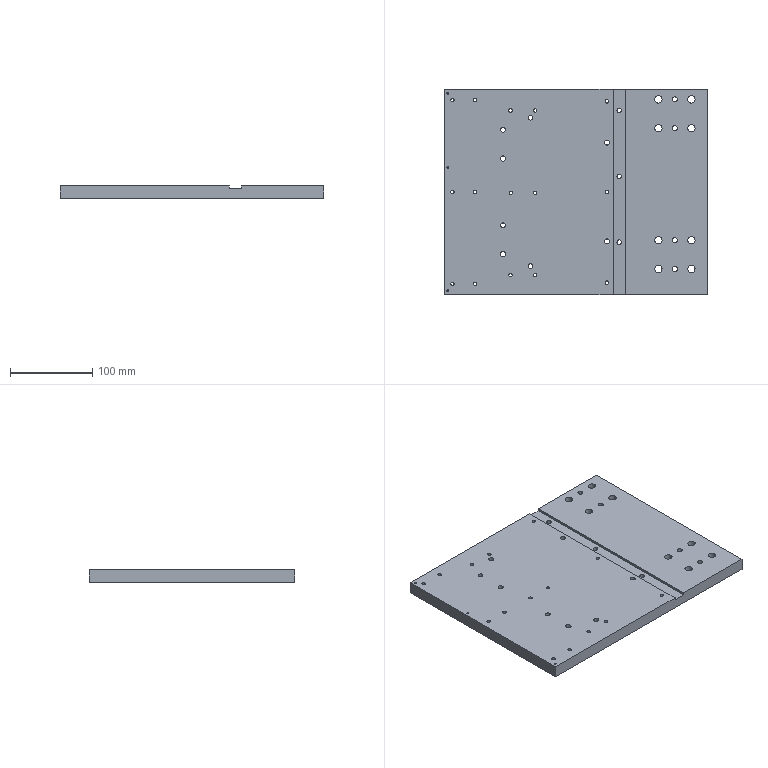Part | 1 solid | 129 faces | box 320 x 250 x 15 mm | volume 1163075 mm3 | cylinder 104 | plane 25 | commonest cylinder face diameters 4.2 x30 6 x24 9 x16 15 x16 2.5 x6 5.5 x6